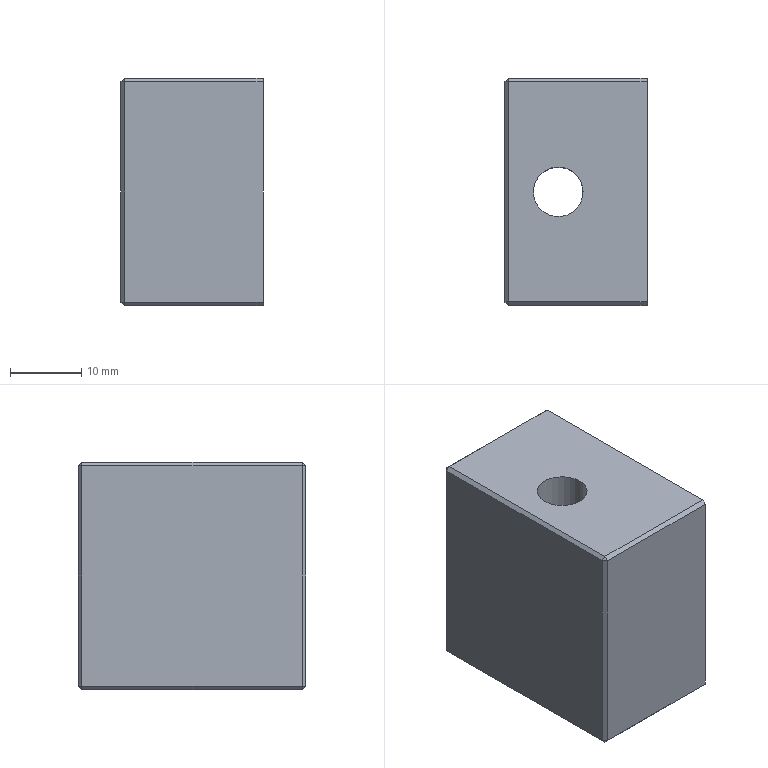Part | STEP file | 02-12 Tensioning block 1 | 1 solid | 26 faces | box 20 x 32 x 32 mm | volume 16333 mm3 | plane 20 | cylinder 6 | commonest cylinder face diameters 7 x2 20 x2 24 x2